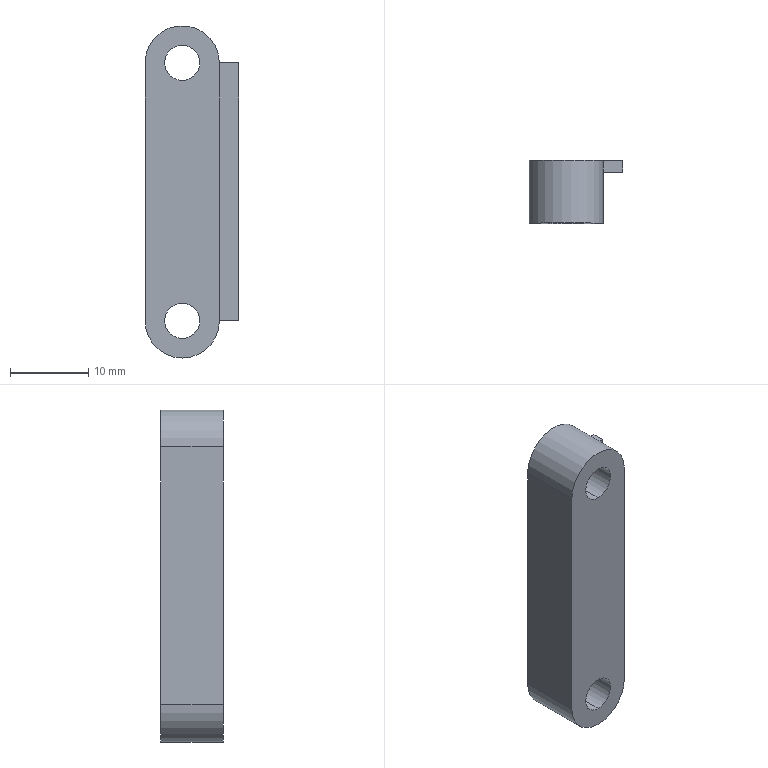Part | SolidWorks | features BaseBody 1 | 1 solid | 21 faces | box 12 x 8 x 42.5 mm | volume 2628 mm3 | cylinder 11 | plane 10 | commonest cylinder face diameters 4.5 x4 8 x4 9.5 x3
STEP:
#1=CARTESIAN_POINT('',(0.,8.,-4.75));
#2=VERTEX_POINT('',#1);
#3=CARTESIAN_POINT('',(-4.75,8.,0.));
#4=VERTEX_POINT('',#3);
#5=CARTESIAN_POINT('',(0.,8.,0.));
#6=DIRECTION('',(0.,1.,0.));
#7=DIRECTION('',(0.,0.,-1.));
#8=AXIS2_PLACEMENT_3D('',#5,#6,#7);
#9=CIRCLE('',#8,4.75);
#10=EDGE_CURVE('',#2,#4,#9,.T.);
#11=ORIENTED_EDGE('',*,*,#10,.F.);
#12=CARTESIAN_POINT('',(0.,0.,-4.75));
#13=VERTEX_POINT('',#12);
#14=CARTESIAN_POINT('',(0.,8.,-4.75));
#15=DIRECTION('',(0.,-1.,0.));
#16=VECTOR('',#15,1000.);
#17=LINE('',#14,#16);
#18=EDGE_CURVE('',#2,#13,#17,.T.);
#19=ORIENTED_EDGE('',*,*,#18,.T.);
#20=CARTESIAN_POINT('',(-4.75,0.,0.));
#21=VERTEX_POINT('',#20);
#22=CARTESIAN_POINT('',(0.,0.,0.));
#23=DIRECTION('',(0.,1.,0.));
#24=DIRECTION('',(0.,0.,-1.));
#25=AXIS2_PLACEMENT_3D('',#22,#23,#24);
#26=CIRCLE('',#25,4.75);
#27=EDGE_CURVE('',#13,#21,#26,.T.);
#28=ORIENTED_EDGE('',*,*,#27,.T.);
#29=CARTESIAN_POINT('',(-4.75,8.,0.));
#30=DIRECTION('',(0.,1.,0.));
#31=VECTOR('',#30,1000.);
#32=LINE('',#29,#31);
#33=EDGE_CURVE('',#21,#4,#32,.T.);
#34=ORIENTED_EDGE('',*,*,#33,.T.);
#35=EDGE_LOOP('',(#11,#19,#28,#34));
#36=FACE_OUTER_BOUND('',#35,.T.);
#37=CARTESIAN_POINT('',(0.,8.,0.));
#38=DIRECTION('',(0.,-1.,0.));
#39=DIRECTION('',(0.,0.,-1.));
#40=AXIS2_PLACEMENT_3D('',#37,#38,#39);
#41=CYLINDRICAL_SURFACE('',#40,4.75);
#42=ADVANCED_FACE('',(#36),#41,.T.);
#43=CARTESIAN_POINT('',(0.,3.4,29.));
#44=VERTEX_POINT('',#43);
#45=CARTESIAN_POINT('',(0.,3.4,37.));
#46=VERTEX_POINT('',#45);
#47=CARTESIAN_POINT('',(0.,3.4,33.));
#48=DIRECTION('',(0.,1.,0.));
#49=DIRECTION('',(0.,0.,1.));
#50=AXIS2_PLACEMENT_3D('',#47,#48,#49);
#51=CIRCLE('',#50,4.);
#52=EDGE_CURVE('',#44,#46,#51,.T.);
#53=ORIENTED_EDGE('',*,*,#52,.F.);
#54=CARTESIAN_POINT('',(0.,8.,29.));
#55=VERTEX_POINT('',#54);
#56=CARTESIAN_POINT('',(0.,8.,29.));
#57=DIRECTION('',(0.,1.,0.));
#58=VECTOR('',#57,1000.);
#59=LINE('',#56,#58);
#60=EDGE_CURVE('',#44,#55,#59,.T.);
#61=ORIENTED_EDGE('',*,*,#60,.T.);
#62=CARTESIAN_POINT('',(0.,8.,37.));
#63=VERTEX_POINT('',#62);
#64=CARTESIAN_POINT('',(0.,8.,33.));
#65=DIRECTION('',(0.,-1.,0.));
#66=DIRECTION('',(0.,0.,1.));
#67=AXIS2_PLACEMENT_3D('',#64,#65,#66);
#68=CIRCLE('',#67,4.);
#69=EDGE_CURVE('',#63,#55,#68,.T.);
#70=ORIENTED_EDGE('',*,*,#69,.F.);
#71=CARTESIAN_POINT('',(0.,8.,37.));
#72=DIRECTION('',(0.,1.,0.));
#73=VECTOR('',#72,1000.);
#74=LINE('',#71,#73);
#75=EDGE_CURVE('',#46,#63,#74,.T.);
#76=ORIENTED_EDGE('',*,*,#75,.F.);
#77=EDGE_LOOP('',(#53,#61,#70,#76));
#78=FACE_OUTER_BOUND('',#77,.T.);
#79=CARTESIAN_POINT('',(0.,8.,33.));
#80=DIRECTION('',(0.,1.,0.));
#81=DIRECTION('',(0.,0.,1.));
#82=AXIS2_PLACEMENT_3D('',#79,#80,#81);
#83=CYLINDRICAL_SURFACE('',#82,4.);
#84=ADVANCED_FACE('',(#78),#83,.F.);
#85=CARTESIAN_POINT('',(0.,3.4,-4.));
#86=VERTEX_POINT('',#85);
#87=CARTESIAN_POINT('',(0.,3.4,4.));
#88=VERTEX_POINT('',#87);
#89=CARTESIAN_POINT('',(0.,3.4,0.));
#90=DIRECTION('',(0.,1.,0.));
#91=DIRECTION('',(0.,0.,1.));
#92=AXIS2_PLACEMENT_3D('',#89,#90,#91);
#93=CIRCLE('',#92,4.);
#94=EDGE_CURVE('',#86,#88,#93,.T.);
#95=ORIENTED_EDGE('',*,*,#94,.F.);
#96=CARTESIAN_POINT('',(0.,8.,-4.));
#97=VERTEX_POINT('',#96);
#98=CARTESIAN_POINT('',(0.,8.,-4.));
#99=DIRECTION('',(0.,1.,0.));
#100=VECTOR('',#99,1000.);
#101=LINE('',#98,#100);
#102=EDGE_CURVE('',#86,#97,#101,.T.);
#103=ORIENTED_EDGE('',*,*,#102,.T.);
#104=CARTESIAN_POINT('',(0.,8.,4.));
#105=VERTEX_POINT('',#104);
#106=CARTESIAN_POINT('',(0.,8.,0.));
#107=DIRECTION('',(0.,-1.,0.));
#108=DIRECTION('',(0.,0.,1.));
#109=AXIS2_PLACEMENT_3D('',#106,#107,#108);
#110=CIRCLE('',#109,4.);
#111=EDGE_CURVE('',#105,#97,#110,.T.);
#112=ORIENTED_EDGE('',*,*,#111,.F.);
#113=CARTESIAN_POINT('',(0.,8.,4.));
#114=DIRECTION('',(0.,1.,0.));
#115=VECTOR('',#114,1000.);
#116=LINE('',#113,#115);
#117=EDGE_CURVE('',#88,#105,#116,.T.);
#118=ORIENTED_EDGE('',*,*,#117,.F.);
#119=EDGE_LOOP('',(#95,#103,#112,#118));
#120=FACE_OUTER_BOUND('',#119,.T.);
#121=CARTESIAN_POINT('',(0.,8.,0.));
#122=DIRECTION('',(0.,1.,0.));
#123=DIRECTION('',(0.,0.,1.));
#124=AXIS2_PLACEMENT_3D('',#121,#122,#123);
#125=CYLINDRICAL_SURFACE('',#124,4.);
#126=ADVANCED_FACE('',(#120),#125,.F.);
#127=CARTESIAN_POINT('',(0.,0.,35.25));
#128=VERTEX_POINT('',#127);
#129=CARTESIAN_POINT('',(0.,0.,30.75));
#130=VERTEX_POINT('',#129);
#131=CARTESIAN_POINT('',(0.,0.,33.));
#132=DIRECTION('',(0.,-1.,0.));
#133=DIRECTION('',(0.,0.,1.));
#134=AXIS2_PLACEMENT_3D('',#131,#132,#133);
#135=CIRCLE('',#134,2.25);
#136=EDGE_CURVE('',#128,#130,#135,.T.);
#137=ORIENTED_EDGE('',*,*,#136,.T.);
#138=CARTESIAN_POINT('',(0.,3.4,30.75));
#139=VERTEX_POINT('',#138);
#140=CARTESIAN_POINT('',(0.,8.,30.75));
#141=DIRECTION('',(0.,1.,0.));
#142=VECTOR('',#141,1000.);
#143=LINE('',#140,#142);
#144=EDGE_CURVE('',#130,#139,#143,.T.);
#145=ORIENTED_EDGE('',*,*,#144,.T.);
#146=CARTESIAN_POINT('',(0.,3.4,35.25));
#147=VERTEX_POINT('',#146);
#148=CARTESIAN_POINT('',(0.,3.4,33.));
#149=DIRECTION('',(0.,1.,0.));
#150=DIRECTION('',(0.,0.,1.));
#151=AXIS2_PLACEMENT_3D('',#148,#149,#150);
#152=CIRCLE('',#151,2.25);
#153=EDGE_CURVE('',#139,#147,#152,.T.);
#154=ORIENTED_EDGE('',*,*,#153,.T.);
#155=CARTESIAN_POINT('',(0.,8.,35.25));
#156=DIRECTION('',(0.,1.,0.));
#157=VECTOR('',#156,1000.);
#158=LINE('',#155,#157);
#159=EDGE_CURVE('',#128,#147,#158,.T.);
#160=ORIENTED_EDGE('',*,*,#159,.F.);
#161=EDGE_LOOP('',(#137,#145,#154,#160));
#162=FACE_OUTER_BOUND('',#161,.T.);
#163=CARTESIAN_POINT('',(0.,8.,33.));
#164=DIRECTION('',(0.,1.,0.));
#165=DIRECTION('',(0.,0.,1.));
#166=AXIS2_PLACEMENT_3D('',#163,#164,#165);
#167=CYLINDRICAL_SURFACE('',#166,2.25);
#168=ADVANCED_FACE('',(#162),#167,.F.);
#169=CARTESIAN_POINT('',(0.,0.,2.25));
#170=VERTEX_POINT('',#169);
#171=CARTESIAN_POINT('',(0.,0.,-2.25));
#172=VERTEX_POINT('',#171);
#173=CARTESIAN_POINT('',(0.,0.,0.));
#174=DIRECTION('',(0.,-1.,0.));
#175=DIRECTION('',(0.,0.,1.));
#176=AXIS2_PLACEMENT_3D('',#173,#174,#175);
#177=CIRCLE('',#176,2.25);
#178=EDGE_CURVE('',#170,#172,#177,.T.);
#179=ORIENTED_EDGE('',*,*,#178,.T.);
#180=CARTESIAN_POINT('',(0.,3.4,-2.25));
#181=VERTEX_POINT('',#180);
#182=CARTESIAN_POINT('',(0.,8.,-2.25));
#183=DIRECTION('',(0.,1.,0.));
#184=VECTOR('',#183,1000.);
#185=LINE('',#182,#184);
#186=EDGE_CURVE('',#172,#181,#185,.T.);
#187=ORIENTED_EDGE('',*,*,#186,.T.);
#188=CARTESIAN_POINT('',(0.,3.4,2.25));
#189=VERTEX_POINT('',#188);
#190=CARTESIAN_POINT('',(0.,3.4,0.));
#191=DIRECTION('',(0.,1.,0.));
#192=DIRECTION('',(0.,0.,1.));
#193=AXIS2_PLACEMENT_3D('',#190,#191,#192);
#194=CIRCLE('',#193,2.25);
#195=EDGE_CURVE('',#181,#189,#194,.T.);
#196=ORIENTED_EDGE('',*,*,#195,.T.);
#197=CARTESIAN_POINT('',(0.,8.,2.25));
#198=DIRECTION('',(0.,1.,0.));
#199=VECTOR('',#198,1000.);
#200=LINE('',#197,#199);
#201=EDGE_CURVE('',#170,#189,#200,.T.);
#202=ORIENTED_EDGE('',*,*,#201,.F.);
#203=EDGE_LOOP('',(#179,#187,#196,#202));
#204=FACE_OUTER_BOUND('',#203,.T.);
#205=CARTESIAN_POINT('',(0.,8.,0.));
#206=DIRECTION('',(0.,1.,0.));
#207=DIRECTION('',(0.,0.,1.));
#208=AXIS2_PLACEMENT_3D('',#205,#206,#207);
#209=CYLINDRICAL_SURFACE('',#208,2.25);
#210=ADVANCED_FACE('',(#204),#209,.F.);
#211=CARTESIAN_POINT('',(7.25,8.,33.));
#212=VERTEX_POINT('',#211);
#213=CARTESIAN_POINT('',(7.25,8.,0.));
#214=VERTEX_POINT('',#213);
#215=CARTESIAN_POINT('',(7.25,8.,0.));
#216=DIRECTION('',(0.,0.,-1.));
#217=VECTOR('',#216,1000.);
#218=LINE('',#215,#217);
#219=EDGE_CURVE('',#212,#214,#218,.T.);
#220=ORIENTED_EDGE('',*,*,#219,.T.);
#221=CARTESIAN_POINT('',(4.75,8.,0.));
#222=VERTEX_POINT('',#221);
#223=CARTESIAN_POINT('',(0.,8.,0.));
#224=DIRECTION('',(-1.,0.,0.));
#225=VECTOR('',#224,1000.);
#226=LINE('',#223,#225);
#227=EDGE_CURVE('',#214,#222,#226,.T.);
#228=ORIENTED_EDGE('',*,*,#227,.T.);
#229=CARTESIAN_POINT('',(0.,8.,0.));
#230=DIRECTION('',(0.,1.,0.));
#231=DIRECTION('',(0.,0.,-1.));
#232=AXIS2_PLACEMENT_3D('',#229,#230,#231);
#233=CIRCLE('',#232,4.75);
#234=EDGE_CURVE('',#222,#2,#233,.T.);
#235=ORIENTED_EDGE('',*,*,#234,.T.);
#236=ORIENTED_EDGE('',*,*,#10,.T.);
#237=CARTESIAN_POINT('',(-4.75,8.,33.));
#238=VERTEX_POINT('',#237);
#239=CARTESIAN_POINT('',(-4.75,8.,0.));
#240=DIRECTION('',(0.,0.,1.));
#241=VECTOR('',#240,1000.);
#242=LINE('',#239,#241);
#243=EDGE_CURVE('',#4,#238,#242,.T.);
#244=ORIENTED_EDGE('',*,*,#243,.T.);
#245=CARTESIAN_POINT('',(4.75,8.,33.));
#246=VERTEX_POINT('',#245);
#247=CARTESIAN_POINT('',(0.,8.,33.));
#248=DIRECTION('',(0.,1.,0.));
#249=DIRECTION('',(0.,0.,-1.));
#250=AXIS2_PLACEMENT_3D('',#247,#248,#249);
#251=CIRCLE('',#250,4.75);
#252=EDGE_CURVE('',#238,#246,#251,.T.);
#253=ORIENTED_EDGE('',*,*,#252,.T.);
#254=CARTESIAN_POINT('',(0.,8.,33.));
#255=DIRECTION('',(1.,0.,0.));
#256=VECTOR('',#255,1000.);
#257=LINE('',#254,#256);
#258=EDGE_CURVE('',#246,#212,#257,.T.);
#259=ORIENTED_EDGE('',*,*,#258,.T.);
#260=EDGE_LOOP('',(#220,#228,#235,#236,#244,#253,#259));
#261=FACE_OUTER_BOUND('',#260,.T.);
#262=ORIENTED_EDGE('',*,*,#69,.T.);
#263=CARTESIAN_POINT('',(0.,8.,33.));
#264=DIRECTION('',(0.,-1.,0.));
#265=DIRECTION('',(0.,0.,1.));
#266=AXIS2_PLACEMENT_3D('',#263,#264,#265);
#267=CIRCLE('',#266,4.);
#268=EDGE_CURVE('',#55,#63,#267,.T.);
#269=ORIENTED_EDGE('',*,*,#268,.T.);
#270=EDGE_LOOP('',(#262,#269));
#271=FACE_BOUND('',#270,.T.);
#272=ORIENTED_EDGE('',*,*,#111,.T.);
#273=CARTESIAN_POINT('',(0.,8.,0.));
#274=DIRECTION('',(0.,-1.,0.));
#275=DIRECTION('',(0.,0.,1.));
#276=AXIS2_PLACEMENT_3D('',#273,#274,#275);
#277=CIRCLE('',#276,4.);
#278=EDGE_CURVE('',#97,#105,#277,.T.);
#279=ORIENTED_EDGE('',*,*,#278,.T.);
#280=EDGE_LOOP('',(#272,#279));
#281=FACE_BOUND('',#280,.T.);
#282=CARTESIAN_POINT('',(0.,8.,0.));
#283=DIRECTION('',(0.,1.,0.));
#284=DIRECTION('',(0.,0.,1.));
#285=AXIS2_PLACEMENT_3D('',#282,#283,#284);
#286=PLANE('',#285);
#287=ADVANCED_FACE('',(#261,#271,#281),#286,.T.);
#288=ORIENTED_EDGE('',*,*,#227,.F.);
#289=CARTESIAN_POINT('',(7.25,6.5,0.));
#290=VERTEX_POINT('',#289);
#291=CARTESIAN_POINT('',(7.25,8.,0.));
#292=DIRECTION('',(0.,1.,0.));
#293=VECTOR('',#292,1000.);
#294=LINE('',#291,#293);
#295=EDGE_CURVE('',#290,#214,#294,.T.);
#296=ORIENTED_EDGE('',*,*,#295,.F.);
#297=CARTESIAN_POINT('',(4.75,6.5,0.));
#298=VERTEX_POINT('',#297);
#299=CARTESIAN_POINT('',(7.25,6.5,0.));
#300=DIRECTION('',(1.,0.,0.));
#301=VECTOR('',#300,1000.);
#302=LINE('',#299,#301);
#303=EDGE_CURVE('',#298,#290,#302,.T.);
#304=ORIENTED_EDGE('',*,*,#303,.F.);
#305=CARTESIAN_POINT('',(4.75,8.,0.));
#306=DIRECTION('',(0.,-1.,0.));
#307=VECTOR('',#306,1000.);
#308=LINE('',#305,#307);
#309=EDGE_CURVE('',#222,#298,#308,.T.);
#310=ORIENTED_EDGE('',*,*,#309,.F.);
#311=EDGE_LOOP('',(#288,#296,#304,#310));
#312=FACE_OUTER_BOUND('',#311,.T.);
#313=CARTESIAN_POINT('',(7.25,8.,0.));
#314=DIRECTION('',(0.,0.,1.));
#315=DIRECTION('',(1.,0.,0.));
#316=AXIS2_PLACEMENT_3D('',#313,#314,#315);
#317=PLANE('',#316);
#318=ADVANCED_FACE('',(#312),#317,.F.);
#319=ORIENTED_EDGE('',*,*,#295,.T.);
#320=ORIENTED_EDGE('',*,*,#219,.F.);
#321=CARTESIAN_POINT('',(7.25,6.5,33.));
#322=VERTEX_POINT('',#321);
#323=CARTESIAN_POINT('',(7.25,0.,33.));
#324=DIRECTION('',(0.,-1.,0.));
#325=VECTOR('',#324,1000.);
#326=LINE('',#323,#325);
#327=EDGE_CURVE('',#212,#322,#326,.T.);
#328=ORIENTED_EDGE('',*,*,#327,.T.);
#329=CARTESIAN_POINT('',(7.25,6.5,0.));
#330=DIRECTION('',(0.,0.,-1.));
#331=VECTOR('',#330,1000.);
#332=LINE('',#329,#331);
#333=EDGE_CURVE('',#322,#290,#332,.T.);
#334=ORIENTED_EDGE('',*,*,#333,.T.);
#335=EDGE_LOOP('',(#319,#320,#328,#334));
#336=FACE_OUTER_BOUND('',#335,.T.);
#337=CARTESIAN_POINT('',(7.25,0.,0.));
#338=DIRECTION('',(1.,0.,0.));
#339=DIRECTION('',(0.,0.,-1.));
#340=AXIS2_PLACEMENT_3D('',#337,#338,#339);
#341=PLANE('',#340);
#342=ADVANCED_FACE('',(#336),#341,.T.);
#343=CARTESIAN_POINT('',(4.75,6.5,33.));
#344=VERTEX_POINT('',#343);
#345=CARTESIAN_POINT('',(7.25,6.5,33.));
#346=DIRECTION('',(-1.,0.,0.));
#347=VECTOR('',#346,1000.);
#348=LINE('',#345,#347);
#349=EDGE_CURVE('',#322,#344,#348,.T.);
#350=ORIENTED_EDGE('',*,*,#349,.F.);
#351=ORIENTED_EDGE('',*,*,#327,.F.);
#352=ORIENTED_EDGE('',*,*,#258,.F.);
#353=CARTESIAN_POINT('',(4.75,8.,33.));
#354=DIRECTION('',(0.,1.,0.));
#355=VECTOR('',#354,1000.);
#356=LINE('',#353,#355);
#357=EDGE_CURVE('',#344,#246,#356,.T.);
#358=ORIENTED_EDGE('',*,*,#357,.F.);
#359=EDGE_LOOP('',(#350,#351,#352,#358));
#360=FACE_OUTER_BOUND('',#359,.T.);
#361=CARTESIAN_POINT('',(7.25,8.,33.));
#362=DIRECTION('',(0.,0.,-1.));
#363=DIRECTION('',(-1.,0.,0.));
#364=AXIS2_PLACEMENT_3D('',#361,#362,#363);
#365=PLANE('',#364);
#366=ADVANCED_FACE('',(#360),#365,.F.);
#367=ORIENTED_EDGE('',*,*,#252,.F.);
#368=CARTESIAN_POINT('',(-4.75,0.,33.));
#369=VERTEX_POINT('',#368);
#370=CARTESIAN_POINT('',(-4.75,8.,33.));
#371=DIRECTION('',(0.,-1.,0.));
#372=VECTOR('',#371,1000.);
#373=LINE('',#370,#372);
#374=EDGE_CURVE('',#238,#369,#373,.T.);
#375=ORIENTED_EDGE('',*,*,#374,.T.);
#376=CARTESIAN_POINT('',(4.75,0.,33.));
#377=VERTEX_POINT('',#376);
#378=CARTESIAN_POINT('',(0.,0.,33.));
#379=DIRECTION('',(0.,1.,0.));
#380=DIRECTION('',(0.,0.,-1.));
#381=AXIS2_PLACEMENT_3D('',#378,#379,#380);
#382=CIRCLE('',#381,4.75);
#383=EDGE_CURVE('',#369,#377,#382,.T.);
#384=ORIENTED_EDGE('',*,*,#383,.T.);
#385=CARTESIAN_POINT('',(4.75,8.,33.));
#386=DIRECTION('',(0.,1.,0.));
#387=VECTOR('',#386,1000.);
#388=LINE('',#385,#387);
#389=EDGE_CURVE('',#377,#344,#388,.T.);
#390=ORIENTED_EDGE('',*,*,#389,.T.);
#391=ORIENTED_EDGE('',*,*,#357,.T.);
#392=EDGE_LOOP('',(#367,#375,#384,#390,#391));
#393=FACE_OUTER_BOUND('',#392,.T.);
#394=CARTESIAN_POINT('',(0.,8.,33.));
#395=DIRECTION('',(0.,-1.,0.));
#396=DIRECTION('',(0.,0.,-1.));
#397=AXIS2_PLACEMENT_3D('',#394,#395,#396);
#398=CYLINDRICAL_SURFACE('',#397,4.75);
#399=ADVANCED_FACE('',(#393),#398,.T.);
#400=ORIENTED_EDGE('',*,*,#374,.F.);
#401=ORIENTED_EDGE('',*,*,#243,.F.);
#402=ORIENTED_EDGE('',*,*,#33,.F.);
#403=CARTESIAN_POINT('',(-4.75,0.,0.));
#404=DIRECTION('',(0.,0.,-1.));
#405=VECTOR('',#404,1000.);
#406=LINE('',#403,#405);
#407=EDGE_CURVE('',#369,#21,#406,.T.);
#408=ORIENTED_EDGE('',*,*,#407,.F.);
#409=EDGE_LOOP('',(#400,#401,#402,#408));
#410=FACE_OUTER_BOUND('',#409,.T.);
#411=CARTESIAN_POINT('',(-4.75,8.,0.));
#412=DIRECTION('',(1.,0.,0.));
#413=DIRECTION('',(0.,0.,-1.));
#414=AXIS2_PLACEMENT_3D('',#411,#412,#413);
#415=PLANE('',#414);
#416=ADVANCED_FACE('',(#410),#415,.F.);
#417=ORIENTED_EDGE('',*,*,#18,.F.);
#418=ORIENTED_EDGE('',*,*,#234,.F.);
#419=ORIENTED_EDGE('',*,*,#309,.T.);
#420=CARTESIAN_POINT('',(4.75,0.,0.));
#421=VERTEX_POINT('',#420);
#422=CARTESIAN_POINT('',(4.75,8.,0.));
#423=DIRECTION('',(0.,-1.,0.));
#424=VECTOR('',#423,1000.);
#425=LINE('',#422,#424);
#426=EDGE_CURVE('',#298,#421,#425,.T.);
#427=ORIENTED_EDGE('',*,*,#426,.T.);
#428=CARTESIAN_POINT('',(0.,0.,0.));
#429=DIRECTION('',(0.,1.,0.));
#430=DIRECTION('',(0.,0.,-1.));
#431=AXIS2_PLACEMENT_3D('',#428,#429,#430);
#432=CIRCLE('',#431,4.75);
#433=EDGE_CURVE('',#421,#13,#432,.T.);
#434=ORIENTED_EDGE('',*,*,#433,.T.);
#435=EDGE_LOOP('',(#417,#418,#419,#427,#434));
#436=FACE_OUTER_BOUND('',#435,.T.);
#437=CARTESIAN_POINT('',(0.,8.,0.));
#438=DIRECTION('',(0.,-1.,0.));
#439=DIRECTION('',(0.,0.,-1.));
#440=AXIS2_PLACEMENT_3D('',#437,#438,#439);
#441=CYLINDRICAL_SURFACE('',#440,4.75);
#442=ADVANCED_FACE('',(#436),#441,.T.);
#443=ORIENTED_EDGE('',*,*,#60,.F.);
#444=CARTESIAN_POINT('',(0.,3.4,33.));
#445=DIRECTION('',(0.,1.,0.));
#446=DIRECTION('',(0.,0.,1.));
#447=AXIS2_PLACEMENT_3D('',#444,#445,#446);
#448=CIRCLE('',#447,4.);
#449=EDGE_CURVE('',#46,#44,#448,.T.);
#450=ORIENTED_EDGE('',*,*,#449,.F.);
#451=ORIENTED_EDGE('',*,*,#75,.T.);
#452=ORIENTED_EDGE('',*,*,#268,.F.);
#453=EDGE_LOOP('',(#443,#450,#451,#452));
#454=FACE_OUTER_BOUND('',#453,.T.);
#455=CARTESIAN_POINT('',(0.,8.,33.));
#456=DIRECTION('',(0.,1.,0.));
#457=DIRECTION('',(0.,0.,1.));
#458=AXIS2_PLACEMENT_3D('',#455,#456,#457);
#459=CYLINDRICAL_SURFACE('',#458,4.);
#460=ADVANCED_FACE('',(#454),#459,.F.);
#461=ORIENTED_EDGE('',*,*,#102,.F.);
#462=CARTESIAN_POINT('',(0.,3.4,0.));
#463=DIRECTION('',(0.,1.,0.));
#464=DIRECTION('',(0.,0.,1.));
#465=AXIS2_PLACEMENT_3D('',#462,#463,#464);
#466=CIRCLE('',#465,4.);
#467=EDGE_CURVE('',#88,#86,#466,.T.);
#468=ORIENTED_EDGE('',*,*,#467,.F.);
#469=ORIENTED_EDGE('',*,*,#117,.T.);
#470=ORIENTED_EDGE('',*,*,#278,.F.);
#471=EDGE_LOOP('',(#461,#468,#469,#470));
#472=FACE_OUTER_BOUND('',#471,.T.);
#473=CARTESIAN_POINT('',(0.,8.,0.));
#474=DIRECTION('',(0.,1.,0.));
#475=DIRECTION('',(0.,0.,1.));
#476=AXIS2_PLACEMENT_3D('',#473,#474,#475);
#477=CYLINDRICAL_SURFACE('',#476,4.);
#478=ADVANCED_FACE('',(#472),#477,.F.);
#479=ORIENTED_EDGE('',*,*,#303,.T.);
#480=ORIENTED_EDGE('',*,*,#333,.F.);
#481=ORIENTED_EDGE('',*,*,#349,.T.);
#482=CARTESIAN_POINT('',(4.75,6.5,33.));
#483=DIRECTION('',(0.,0.,1.));
#484=VECTOR('',#483,1000.);
#485=LINE('',#482,#484);
#486=EDGE_CURVE('',#298,#344,#485,.T.);
#487=ORIENTED_EDGE('',*,*,#486,.F.);
#488=EDGE_LOOP('',(#479,#480,#481,#487));
#489=FACE_OUTER_BOUND('',#488,.T.);
#490=CARTESIAN_POINT('',(7.25,6.5,33.));
#491=DIRECTION('',(0.,1.,0.));
#492=DIRECTION('',(0.,0.,1.));
#493=AXIS2_PLACEMENT_3D('',#490,#491,#492);
#494=PLANE('',#493);
#495=ADVANCED_FACE('',(#489),#494,.F.);
#496=ORIENTED_EDGE('',*,*,#389,.F.);
#497=CARTESIAN_POINT('',(4.75,0.,0.));
#498=DIRECTION('',(0.,0.,1.));
#499=VECTOR('',#498,1000.);
#500=LINE('',#497,#499);
#501=EDGE_CURVE('',#421,#377,#500,.T.);
#502=ORIENTED_EDGE('',*,*,#501,.F.);
#503=ORIENTED_EDGE('',*,*,#426,.F.);
#504=ORIENTED_EDGE('',*,*,#486,.T.);
#505=EDGE_LOOP('',(#496,#502,#503,#504));
#506=FACE_OUTER_BOUND('',#505,.T.);
#507=CARTESIAN_POINT('',(4.75,8.,0.));
#508=DIRECTION('',(-1.,0.,0.));
#509=DIRECTION('',(0.,0.,1.));
#510=AXIS2_PLACEMENT_3D('',#507,#508,#509);
#511=PLANE('',#510);
#512=ADVANCED_FACE('',(#506),#511,.F.);
#513=ORIENTED_EDGE('',*,*,#501,.T.);
#514=ORIENTED_EDGE('',*,*,#383,.F.);
#515=ORIENTED_EDGE('',*,*,#407,.T.);
#516=ORIENTED_EDGE('',*,*,#27,.F.);
#517=ORIENTED_EDGE('',*,*,#433,.F.);
#518=EDGE_LOOP('',(#513,#514,#515,#516,#517));
#519=FACE_OUTER_BOUND('',#518,.T.);
#520=ORIENTED_EDGE('',*,*,#136,.F.);
#521=CARTESIAN_POINT('',(0.,0.,33.));
#522=DIRECTION('',(0.,-1.,0.));
#523=DIRECTION('',(0.,0.,1.));
#524=AXIS2_PLACEMENT_3D('',#521,#522,#523);
#525=CIRCLE('',#524,2.25);
#526=EDGE_CURVE('',#130,#128,#525,.T.);
#527=ORIENTED_EDGE('',*,*,#526,.F.);
#528=EDGE_LOOP('',(#520,#527));
#529=FACE_BOUND('',#528,.T.);
#530=ORIENTED_EDGE('',*,*,#178,.F.);
#531=CARTESIAN_POINT('',(0.,0.,0.));
#532=DIRECTION('',(0.,-1.,0.));
#533=DIRECTION('',(0.,0.,1.));
#534=AXIS2_PLACEMENT_3D('',#531,#532,#533);
#535=CIRCLE('',#534,2.25);
#536=EDGE_CURVE('',#172,#170,#535,.T.);
#537=ORIENTED_EDGE('',*,*,#536,.F.);
#538=EDGE_LOOP('',(#530,#537));
#539=FACE_BOUND('',#538,.T.);
#540=CARTESIAN_POINT('',(0.,0.,0.));
#541=DIRECTION('',(0.,1.,0.));
#542=DIRECTION('',(0.,0.,1.));
#543=AXIS2_PLACEMENT_3D('',#540,#541,#542);
#544=PLANE('',#543);
#545=ADVANCED_FACE('',(#519,#529,#539),#544,.F.);
#546=ORIENTED_EDGE('',*,*,#449,.T.);
#547=ORIENTED_EDGE('',*,*,#52,.T.);
#548=EDGE_LOOP('',(#546,#547));
#549=FACE_OUTER_BOUND('',#548,.T.);
#550=CARTESIAN_POINT('',(0.,3.4,33.));
#551=DIRECTION('',(0.,1.,0.));
#552=DIRECTION('',(0.,0.,1.));
#553=AXIS2_PLACEMENT_3D('',#550,#551,#552);
#554=CIRCLE('',#553,2.25);
#555=EDGE_CURVE('',#147,#139,#554,.T.);
#556=ORIENTED_EDGE('',*,*,#555,.F.);
#557=ORIENTED_EDGE('',*,*,#153,.F.);
#558=EDGE_LOOP('',(#556,#557));
#559=FACE_BOUND('',#558,.T.);
#560=CARTESIAN_POINT('',(2.25,3.4,33.));
#561=DIRECTION('',(0.,-1.,0.));
#562=DIRECTION('',(0.,0.,-1.));
#563=AXIS2_PLACEMENT_3D('',#560,#561,#562);
#564=PLANE('',#563);
#565=ADVANCED_FACE('',(#549,#559),#564,.F.);
#566=ORIENTED_EDGE('',*,*,#467,.T.);
#567=ORIENTED_EDGE('',*,*,#94,.T.);
#568=EDGE_LOOP('',(#566,#567));
#569=FACE_OUTER_BOUND('',#568,.T.);
#570=CARTESIAN_POINT('',(0.,3.4,0.));
#571=DIRECTION('',(0.,1.,0.));
#572=DIRECTION('',(0.,0.,1.));
#573=AXIS2_PLACEMENT_3D('',#570,#571,#572);
#574=CIRCLE('',#573,2.25);
#575=EDGE_CURVE('',#189,#181,#574,.T.);
#576=ORIENTED_EDGE('',*,*,#575,.F.);
#577=ORIENTED_EDGE('',*,*,#195,.F.);
#578=EDGE_LOOP('',(#576,#577));
#579=FACE_BOUND('',#578,.T.);
#580=CARTESIAN_POINT('',(2.25,3.4,0.));
#581=DIRECTION('',(0.,-1.,0.));
#582=DIRECTION('',(0.,0.,-1.));
#583=AXIS2_PLACEMENT_3D('',#580,#581,#582);
#584=PLANE('',#583);
#585=ADVANCED_FACE('',(#569,#579),#584,.F.);
#586=ORIENTED_EDGE('',*,*,#144,.F.);
#587=ORIENTED_EDGE('',*,*,#526,.T.);
#588=ORIENTED_EDGE('',*,*,#159,.T.);
#589=ORIENTED_EDGE('',*,*,#555,.T.);
#590=EDGE_LOOP('',(#586,#587,#588,#589));
#591=FACE_OUTER_BOUND('',#590,.T.);
#592=CARTESIAN_POINT('',(0.,8.,33.));
#593=DIRECTION('',(0.,1.,0.));
#594=DIRECTION('',(0.,0.,1.));
#595=AXIS2_PLACEMENT_3D('',#592,#593,#594);
#596=CYLINDRICAL_SURFACE('',#595,2.25);
#597=ADVANCED_FACE('',(#591),#596,.F.);
#598=ORIENTED_EDGE('',*,*,#186,.F.);
#599=ORIENTED_EDGE('',*,*,#536,.T.);
#600=ORIENTED_EDGE('',*,*,#201,.T.);
#601=ORIENTED_EDGE('',*,*,#575,.T.);
#602=EDGE_LOOP('',(#598,#599,#600,#601));
#603=FACE_OUTER_BOUND('',#602,.T.);
#604=CARTESIAN_POINT('',(0.,8.,0.));
#605=DIRECTION('',(0.,1.,0.));
#606=DIRECTION('',(0.,0.,1.));
#607=AXIS2_PLACEMENT_3D('',#604,#605,#606);
#608=CYLINDRICAL_SURFACE('',#607,2.25);
#609=ADVANCED_FACE('',(#603),#608,.F.);
#610=CLOSED_SHELL('',(#42,#84,#126,#168,#210,#287,#318,#342,#366,#399,#416,#442,#460,#478,#495,#512,#545,#565,#585,#597,#609));
#611=MANIFOLD_SOLID_BREP('',#610);
#612=CARTESIAN_POINT('',(0.,0.,0.));
#613=DIRECTION('',(0.,0.,1.));
#614=DIRECTION('',(1.,0.,0.));
#615=AXIS2_PLACEMENT_3D('',#612,#613,#614);
#616=(LENGTH_UNIT()NAMED_UNIT(*)SI_UNIT(.MILLI.,.METRE.));
#617=UNCERTAINTY_MEASURE_WITH_UNIT(LENGTH_MEASURE(0.00001),#616,'','');
#618=(NAMED_UNIT(*)PLANE_ANGLE_UNIT()SI_UNIT($,.RADIAN.));
#619=(NAMED_UNIT(*)SI_UNIT($,.STERADIAN.)SOLID_ANGLE_UNIT());
#620=(GEOMETRIC_REPRESENTATION_CONTEXT(3)GLOBAL_UNCERTAINTY_ASSIGNED_CONTEXT((#617))GLOBAL_UNIT_ASSIGNED_CONTEXT((#616,#618,#619))REPRESENTATION_CONTEXT('',''));
#621=ADVANCED_BREP_SHAPE_REPRESENTATION('',(#611,#615),#620);